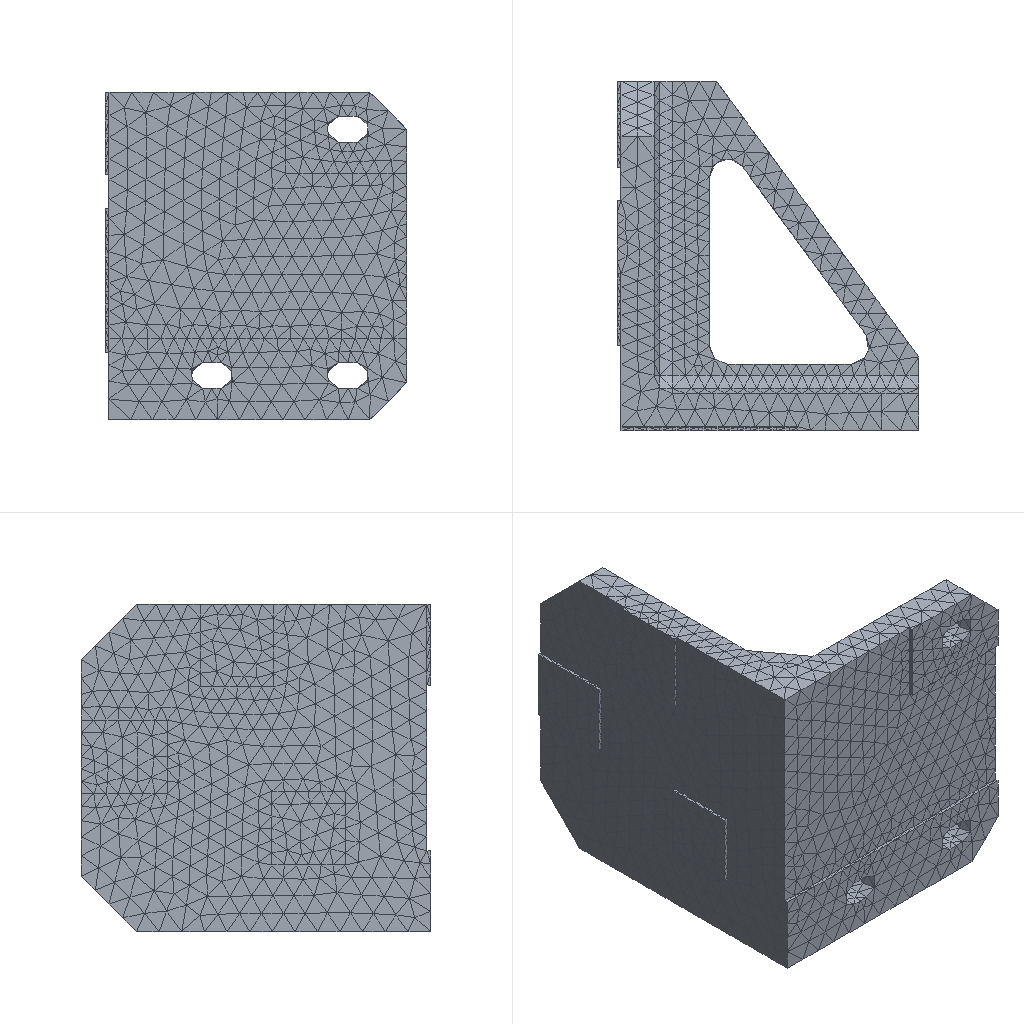Simulation study | nx simcenter
Set-up summary:
category,name,step,type,value,unit,region
solver,nx_nastran (Simcenter)
units,not stated in the deck,,not stated
analysis,deck,,static,static
analysis,solution,,SOL,101
load_step,SUBCASE 1,1,SUBCASE,SPC=1 LOAD=2
load_step,requested,,,1
mesh,nodes,,,16965
mesh,elements,,,9346
element_type,CTETRA,,solid,9346
load,nodal force total,,FX,5999999.98,model units
load,nodal force total,,FY,0.0,model units
load,nodal force total,,FZ,0.0,model units
load,load commands in deck,,count,292
bc,support commands in deck,,count,587
analysis,NX solution 0,,Structural,Linear Statics - Single Constraint
check,setup vs results,,match,every grid point's frame and coordinates and every element id; grid points of CTETRA elements
Nastran input file, long lists of numbers shortened:
$*$$$$$$$$$$$$$$$$$$$$$$$$$$$$$$$$$$$$$$$$$$$$$$$$$$$$$$$$$$$$$$$$$
$*
$*                    NX v10.0.0.24 TRANSLATOR
$*                    FOR NX NASTRAN VERSION 10.0
$ (33 more lines like these left out)
ASSIGN OUTPUT2='155_sim1-solution_1.op2' UNIT=12
$*
$*$$$$$$$$$$$$$$$$$$$$$$$$$$$$$$$$$$$
$*
$* EXECUTIVE CONTROL
$*
$*$$$$$$$$$$$$$$$$$$$$$$$$$$$$$$$$$$$
$*
ID,NASTRAN,155_sim1-solution_1
SOL 101
CEND
$*
$*$$$$$$$$$$$$$$$$$$$$$$$$$$$$$$$$$$$
$*
$* CASE CONTROL
$*
$*$$$$$$$$$$$$$$$$$$$$$$$$$$$$$$$$$$$
$*
TITLE = Solution 1
ECHO = NONE
SPC = 1
OUTPUT
BCRESULTS(TRACTION,FORCE,PLOT) = ALL
DISPLACEMENT(PLOT) = ALL
ESE(PLOT) = ALL
FORCE(PLOT,CORNER) = ALL
OLOAD(PLOT) = ALL
SPCFORCES(PLOT) = ALL
STRAIN(PLOT,FIBER,CORNER) = ALL
STRESS(PLOT,CORNER) = ALL
$*  NX Step: Subcase - Static Loads 1
SUBCASE 1
LABEL = Subcase - Static Loads 1
LOAD = 2
$*
$*$$$$$$$$$$$$$$$$$$$$$$$$$$$$$$$$$$$
$*
$* BULK DATA
$*
$*$$$$$$$$$$$$$$$$$$$$$$$$$$$$$$$$$$$
$*
BEGIN BULK
$*
$* PARAM CARDS
$*
PARAM      K6ROT100.0000
PARAM     OIBULK     YES
PARAM    OMACHPR     YES
PARAM       POST      -2
PARAM    POSTEXT     YES
PARAM    UNITSYS   MN-MM
$*
$* GRID CARDS
$*
GRID*              16856               03.0000000000E+002.8180194855E+01+
*       2.8609146118E+01               0
GRID*              16857               03.0000000000E+002.8180194855E+01+
*       8.6091451645E+00               0
$ (33926 more lines like these left out)
$*
$* ELEMENT CARDS
$*
$*  NX Mesh Collector: Solid(1)
$*  NX Mesh: 3d_mesh(1)
CTETRA         1       1       1    8775    8777   15348     560    9242+
+            561     562    9244    9247
CTETRA         2       1       1       2       3       4     563     564+
+            565     566     567     568
$ (18688 more lines like these left out)
$*
$* PROPERTY CARDS
$*
$*  NX Property: PSOLID1
PSOLID         1       1       0                           SMECH
$*
$* MATERIAL CARDS
$*
$*  NX Material: 2A12
MAT1           17.3119+7        0.3300002.8000-62.1355-5
MATT1          1       1               2               3
TABLEM1        1                                                        +
+        20.00007.3119+7 21.11007.3119+7 23.89007.3119+7 37.78007.3119+7+
+        51.67007.3119+7 65.56007.2429+7 79.44007.2429+7 93.33007.1739+7+
+       107.22007.1049+7121.11007.0359+7135.00006.9670+7148.89006.8980+7+
+       162.78006.8290+7176.67006.6910+7190.56006.6221+7204.44006.4841+7+
+       218.33006.3461+7232.22006.1392+7246.11006.0012+7260.00005.8633+7+
+       273.89005.7253+7287.78005.5184+7301.67005.3804+7315.56005.1735+7+
+       329.44004.9665+7343.33004.7596+7357.22004.6216+7371.11004.4147+7+
+           ENDT
TABLEM1        2                                                        +
+        20.00000.330000 21.11000.330000    ENDT
TABLEM1        3                                                        +
+        20.00002.1600-5 93.33002.2500-5107.22002.2662-5121.11002.2824-5+
+       135.00002.2968-5148.89002.3130-5162.78002.3274-5176.67002.3418-5+
+       190.56002.3544-5204.44002.3688-5218.33002.3814-5232.22002.3958-5+
+       246.11002.4066-5260.00002.4192-5273.89002.4300-5287.78002.4408-5+
+       301.67002.4498-5315.56002.4606-5329.44002.4696-5343.33002.4786-5+
+       357.22002.4876-5371.11002.4984-5385.00002.5110-5398.89002.5254-5+
+       412.78002.5398-5426.67002.5560-5    ENDT
$*
$* LOAD AND CONSTRAINT CARDS
$*
$*  NX Load and Constraint: Fixed(1)
SPC            1   13105  123456  0.0000
SPC            1   13106  123456  0.0000
SPC            1   13107  123456  0.0000
SPC            1   13108  123456  0.0000
$ (583 more lines like these left out)
$*  NX Load and Constraint: Force(1)
FORCE          2    8307       020101.551.000000  0.0000  0.0000
FORCE          2    8308       023124.151.000000  0.0000  0.0000
FORCE          2    8309       025886.031.000000  0.0000  0.0000
FORCE          2    8310       031722.381.000000  0.0000  0.0000
$ (288 more lines like these left out)
ENDDATA d4abd089
Results summary:
result,analysis,,,static
result,last_loadstep,,,1
result,primary field,,,displacements
result,reaction total,,FX,-6000002.5,model units
result,reaction total,,FY,1.6,model units
result,reaction total,,FZ,1.567,model units
result,NX solution 0,,loadcases,1,mm